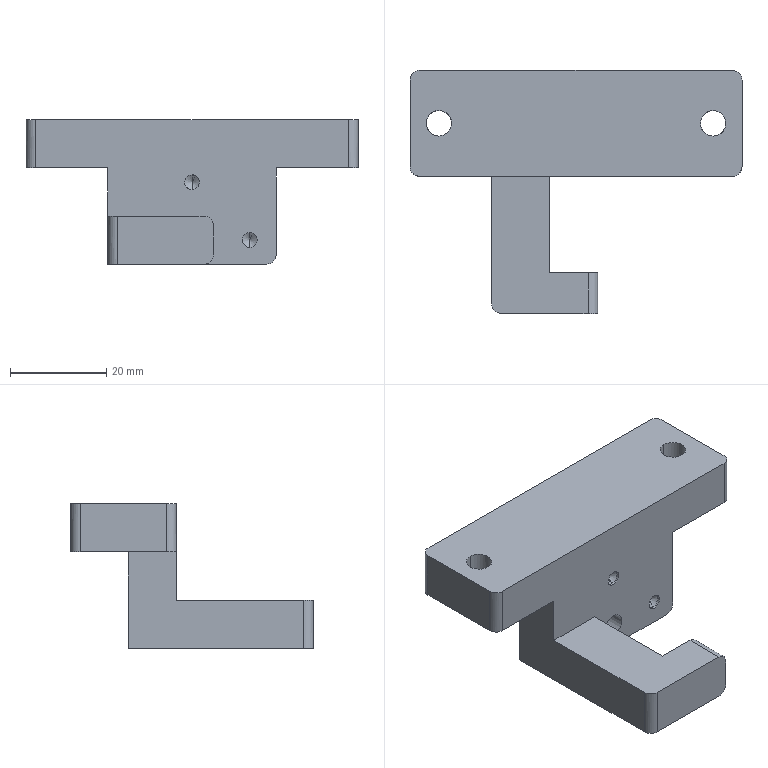NC program | NX | posted with a generic post | part box 69 x 50.5 x 30 mm
Whole program:
N10 G17 G21 G94 G90
(ZLEVEL_PROFILE_1 , TOOL : D10JING)
N12 T14 M6
N14 G54
N16 G17 G0 G90 X-34.145 Y32.098 B0. C0. S9500 M3
N18 G43 Z30. H14
N20 Z-13.5
N22 G94 G1 Z-15. F1000.
N24 X-33.366 Y30.75
N26 G3 X-32.5 Y30.25 R1.
N28 G1 X32.5 F1500.
N30 G2 X39.5 Y23.25 R7.
N32 G1 Y5.25
N34 G2 X32.5 Y-1.75 R7.
N36 G1 X-0.5
N38 Y-11.75
N40 X4.506
N42 G2 X9.5 Y-16.752 R4.998
N44 G1 Y-25.25
N46 G2 X4.5 Y-30.25 R5.
N48 G1 X-15.5
N50 G2 X-22.5 Y-23.25 R7.
N52 G1 Y-1.75
N54 X-32.5
N56 G2 X-39.5 Y5.25 R7.
N58 G1 Y23.25
N60 G2 X-32.5 Y30.25 R7.
N62 G1 X32.5 Z-18.486
N64 X32.866 Y30.24 Z-18.506
N66 X33.232 Y30.212 Z-18.526
N68 X33.595 Y30.164 Z-18.545
N70 X33.955 Y30.097 Z-18.565
N72 X34.312 Y30.011 Z-18.585
N74 X34.663 Y29.907 Z-18.604
N76 X35.009 Y29.785 Z-18.624
N78 X35.347 Y29.645 Z-18.644
N80 X35.678 Y29.487 Z-18.663
N82 X36. Y29.312 Z-18.683
N84 X36.312 Y29.121 Z-18.703
N86 X36.614 Y28.913 Z-18.722
N88 X36.905 Y28.69 Z-18.742
N90 X37.184 Y28.452 Z-18.762
N92 X37.45 Y28.2 Z-18.781
N94 X37.702 Y27.934 Z-18.801
N96 X37.94 Y27.655 Z-18.821
N98 X38.163 Y27.364 Z-18.84
N100 X38.371 Y27.062 Z-18.86
N102 X38.562 Y26.75 Z-18.879
N104 X38.737 Y26.428 Z-18.899
N106 X38.895 Y26.097 Z-18.919
N108 X39.035 Y25.759 Z-18.938
N110 X39.157 Y25.413 Z-18.958
N112 X39.261 Y25.062 Z-18.978
N114 X39.347 Y24.705 Z-18.997
N116 X39.414 Y24.345 Z-19.017
N118 X39.462 Y23.982 Z-19.037
N120 X39.49 Y23.616 Z-19.056
N122 X39.5 Y23.25 Z-19.076
N124 Y5.25 Z-20.041
N126 X39.49 Y4.884 Z-20.061
N128 X39.462 Y4.518 Z-20.081
N130 X39.414 Y4.155 Z-20.1
N132 X39.347 Y3.795 Z-20.12
N134 X39.261 Y3.438 Z-20.14
N136 X39.157 Y3.087 Z-20.159
N138 X39.035 Y2.741 Z-20.179
N140 X38.895 Y2.403 Z-20.199
N142 X38.737 Y2.072 Z-20.218
N144 X38.562 Y1.75 Z-20.238
N146 X38.371 Y1.438 Z-20.258
N148 X38.163 Y1.136 Z-20.277
N150 X37.94 Y0.845 Z-20.297
N152 X37.702 Y0.566 Z-20.317
N154 X37.45 Y0.3 Z-20.336
N156 X37.184 Y0.048 Z-20.356
N158 X36.905 Y-0.19 Z-20.376
N160 X36.614 Y-0.413 Z-20.395
N162 X36.312 Y-0.621 Z-20.415
N164 X36. Y-0.812 Z-20.434
N166 X35.678 Y-0.987 Z-20.454
N168 X35.347 Y-1.145 Z-20.474
N170 X35.009 Y-1.285 Z-20.493
N172 X34.663 Y-1.407 Z-20.513
N174 X34.312 Y-1.511 Z-20.533
N176 X33.955 Y-1.597 Z-20.552
N178 X33.595 Y-1.664 Z-20.572
N180 X33.232 Y-1.712 Z-20.592
N182 X32.866 Y-1.74 Z-20.611
N184 X32.5 Y-1.75 Z-20.631
N186 X-0.5 Z-22.401
N188 Y-11.75 Z-22.937
N190 X2.004 Z-23.072
N192 X4.507 Z-23.206
N194 X4.808 Y-11.76 Z-23.222
N196 X5.109 Y-11.787 Z-23.238
N198 X5.407 Y-11.833 Z-23.255
N200 X5.702 Y-11.897 Z-23.271
N202 X5.993 Y-11.978 Z-23.287
N204 X6.278 Y-12.077 Z-23.303
N206 X6.557 Y-12.193 Z-23.319
N208 X6.828 Y-12.325 Z-23.335
N210 X7.091 Y-12.474 Z-23.352
N212 X7.344 Y-12.638 Z-23.368
N214 X7.587 Y-12.817 Z-23.384
N216 X7.819 Y-13.011 Z-23.4
N218 X8.038 Y-13.218 Z-23.416
N220 X8.245 Y-13.438 Z-23.433
N222 X8.438 Y-13.67 Z-23.449
N224 X8.617 Y-13.913 Z-23.465
N226 X8.781 Y-14.167 Z-23.481
N228 X8.929 Y-14.43 Z-23.497
N230 X9.061 Y-14.701 Z-23.513
N232 X9.176 Y-14.98 Z-23.53
N234 X9.274 Y-15.265 Z-23.546
N236 X9.355 Y-15.556 Z-23.562
N238 X9.418 Y-15.851 Z-23.578
N240 X9.464 Y-16.15 Z-23.594
N242 X9.491 Y-16.45 Z-23.611
N244 X9.5 Y-16.751 Z-23.627
N246 Y-21.001 Z-23.855
N248 Y-25.25 Z-24.083
N250 X9.491 Y-25.552 Z-24.099
N252 X9.464 Y-25.853 Z-24.115
N254 X9.418 Y-26.151 Z-24.131
N256 X9.355 Y-26.447 Z-24.147
N258 X9.274 Y-26.738 Z-24.164
N260 X9.175 Y-27.023 Z-24.18
N262 X9.06 Y-27.302 Z-24.196
N264 X8.927 Y-27.574 Z-24.212
N266 X8.779 Y-27.837 Z-24.228
N268 X8.615 Y-28.09 Z-24.245
N270 X8.436 Y-28.334 Z-24.261
N272 X8.243 Y-28.566 Z-24.277
N274 X8.036 Y-28.786 Z-24.293
N276 X7.816 Y-28.993 Z-24.309
N278 X7.584 Y-29.186 Z-24.325
N280 X7.34 Y-29.365 Z-24.342
N282 X7.087 Y-29.529 Z-24.358
N284 X6.824 Y-29.677 Z-24.374
N286 X6.552 Y-29.81 Z-24.39
N288 X6.273 Y-29.925 Z-24.406
N290 X5.988 Y-30.024 Z-24.423
N292 X5.697 Y-30.105 Z-24.439
N294 X5.401 Y-30.168 Z-24.455
N296 X5.103 Y-30.214 Z-24.471
N298 X4.802 Y-30.241 Z-24.487
N300 X4.5 Y-30.25 Z-24.504
N302 X-15.5 Z-25.576
N304 X-15.866 Y-30.24 Z-25.596
N306 X-16.232 Y-30.212 Z-25.616
N308 X-16.595 Y-30.164 Z-25.635
N310 X-16.955 Y-30.097 Z-25.655
N312 X-17.312 Y-30.011 Z-25.675
N314 X-17.663 Y-29.907 Z-25.694
N316 X-18.009 Y-29.785 Z-25.714
N318 X-18.347 Y-29.645 Z-25.734
N320 X-18.678 Y-29.487 Z-25.753
N322 X-19. Y-29.312 Z-25.773
N324 X-19.312 Y-29.121 Z-25.793
N326 X-19.614 Y-28.913 Z-25.812
N328 X-19.905 Y-28.69 Z-25.832
N330 X-20.184 Y-28.452 Z-25.851
N332 X-20.45 Y-28.2 Z-25.871
N334 X-20.702 Y-27.934 Z-25.891
N336 X-20.94 Y-27.655 Z-25.91
N338 X-21.163 Y-27.364 Z-25.93
N340 X-21.371 Y-27.062 Z-25.95
N342 X-21.562 Y-26.75 Z-25.969
N344 X-21.737 Y-26.428 Z-25.989
N346 X-21.895 Y-26.097 Z-26.009
N348 X-22.035 Y-25.759 Z-26.028
N350 X-22.157 Y-25.413 Z-26.048
N352 X-22.261 Y-25.062 Z-26.068
N354 X-22.347 Y-24.705 Z-26.087
N356 X-22.414 Y-24.345 Z-26.107
N358 X-22.462 Y-23.982 Z-26.127
N360 X-22.49 Y-23.616 Z-26.146
N362 X-22.5 Y-23.25 Z-26.166
N364 Y-1.75 Z-27.319
N366 X-32.5 Z-27.855
N368 X-32.866 Y-1.74 Z-27.875
N370 X-33.232 Y-1.712 Z-27.895
N372 X-33.595 Y-1.664 Z-27.914
N374 X-33.955 Y-1.597 Z-27.934
N376 X-34.312 Y-1.511 Z-27.954
N378 X-34.663 Y-1.407 Z-27.973
N380 X-35.009 Y-1.285 Z-27.993
N382 X-35.347 Y-1.145 Z-28.013
N384 X-35.678 Y-0.987 Z-28.032
N386 X-36. Y-0.812 Z-28.052
N388 X-36.312 Y-0.621 Z-28.072
N390 X-36.614 Y-0.413 Z-28.091
N392 X-36.905 Y-0.19 Z-28.111
N394 X-37.184 Y0.048 Z-28.131
N396 X-37.45 Y0.3 Z-28.15
N398 X-37.702 Y0.566 Z-28.17
N400 X-37.94 Y0.845 Z-28.19
N402 X-38.163 Y1.136 Z-28.209
N404 X-38.371 Y1.438 Z-28.229
N406 X-38.562 Y1.75 Z-28.248
N408 X-38.737 Y2.072 Z-28.268
N410 X-38.895 Y2.403 Z-28.288
N412 X-39.035 Y2.741 Z-28.307
N414 X-39.157 Y3.087 Z-28.327
N416 X-39.261 Y3.438 Z-28.347
N418 X-39.347 Y3.795 Z-28.366
N420 X-39.414 Y4.155 Z-28.386
N422 X-39.462 Y4.518 Z-28.406
N424 X-39.49 Y4.884 Z-28.425
N426 X-39.5 Y5.25 Z-28.445
N428 Y23.25 Z-29.41
N430 X-39.49 Y23.616 Z-29.43
N432 X-39.462 Y23.982 Z-29.45
N434 X-39.414 Y24.345 Z-29.469
N436 X-39.347 Y24.705 Z-29.489
N438 X-39.261 Y25.062 Z-29.509
N440 X-39.157 Y25.413 Z-29.528
N442 X-39.035 Y25.759 Z-29.548
N444 X-38.895 Y26.097 Z-29.568
N446 X-38.737 Y26.428 Z-29.587
N448 X-38.562 Y26.75 Z-29.607
N450 X-38.371 Y27.062 Z-29.627
N452 X-38.163 Y27.364 Z-29.646
N454 X-37.94 Y27.655 Z-29.666
N456 X-37.702 Y27.934 Z-29.686
N458 X-37.45 Y28.2 Z-29.705
N460 X-37.184 Y28.452 Z-29.725
N462 X-36.905 Y28.69 Z-29.745
N464 X-36.614 Y28.913 Z-29.764
N466 X-36.312 Y29.121 Z-29.784
N468 X-36. Y29.312 Z-29.803
N470 X-35.678 Y29.487 Z-29.823
N472 X-35.347 Y29.645 Z-29.843
N474 X-35.009 Y29.785 Z-29.862
N476 X-34.663 Y29.907 Z-29.882
N478 X-34.312 Y30.011 Z-29.902
N480 X-33.955 Y30.097 Z-29.921
N482 X-33.595 Y30.164 Z-29.941
N484 X-33.232 Y30.212 Z-29.961
N486 X-32.866 Y30.24 Z-29.98
N488 X-32.5 Y30.25 Z-30.
N490 X32.5
N492 G2 X39.5 Y23.25 R7.
N494 G1 Y5.25
N496 G2 X32.5 Y-1.75 R7.
N498 G1 X-0.5
N500 Y-11.75
N502 X4.507
N504 G2 X9.5 Y-16.752 R4.998
N506 G1 Y-25.25
N508 G2 X4.5 Y-30.25 R5.
N510 G1 X-15.5
N512 G2 X-22.5 Y-23.25 R7.
N514 G1 Y-1.75
N516 X-32.5
N518 G2 X-39.5 Y5.25 R7.
N520 G1 Y23.25
N522 G2 X-32.5 Y30.25 R7.
N524 G3 X-31.634 Y30.75 R1.
N526 G1 X-30.768 Y32.25
N528 Z-28.5
N530 G0 Z30.
N532 M5
(FLOOR_WALL_1_COPY , TOOL : D6)
N534 T12 M6
N536 G54
N538 G17 G0 G90 X-22. Y-15.362 B0. C0. S9500 M3
N540 G43 Z30. H12
N542 Z-18.5
N544 G94 G1 Z-20. F1200.
N546 X-20.8 Y-14.67
N548 G3 X-20.5 Y-14.15 R0.6
N550 G1 Y-0.05
N552 X-2.5
N554 Y-13.75
N556 X5.5
N558 Y-28.25
N560 X-15.637
N562 X-16.42 Y-28.178
N564 X-17.352 Y-27.91
N566 X-18.247 Y-27.446
N568 X-19.047 Y-26.797
N570 X-19.696 Y-25.997
N572 X-20.16 Y-25.102
N574 X-20.428 Y-24.17
N576 X-20.5 Y-23.387
N578 Y-14.15
N580 X-17.5
N582 Y-3.05
N584 X-5.5
N586 Y-13.75
N588 G3 X-2.5 Y-16.75 R3.
N590 G1 X2.5
N592 Y-25.25
N594 X-15.5
N596 G2 X-17.5 Y-23.25 R2.
N598 G1 Y-14.15
N600 X-14.5
N602 Y-6.05
N604 X-8.5
N606 Y-13.75
N608 G3 X-2.5 Y-19.75 R6.
N610 G1 X-0.5
N612 Y-22.25
N614 X-14.5
N616 Y-14.15
N618 X-11.5
N620 Y-9.05
N622 Y-13.75
N624 G3 X-9.624 Y-19.25 R9.
N626 G1 X-11.5
N628 Y-14.15
N630 G3 X-11.8 Y-13.63 R0.6
N632 G1 Z-18.5
N634 G0 X-1. Y-1.748
N636 G1 Z-20.
N638 X-1.98 Y-0.05
N640 G3 X-2.5 Y0.25 R0.6
N642 G1 X-20.5
N644 G3 X-21.02 Y-0.05 R0.6
N646 G1 X-22. Y-1.748
N648 Z-18.5
N650 G0 Z30.
(PLANAR_MILL_COPY , TOOL : D6A45)
N652 T01 M6
N654 G17 G43 G0 G90 X29.75 Y13.384 Z30. B0. C0. S9500 H1 M3
N656 Z0.5
N658 G94 G1 Z-1. F1250.
N660 G3 X30.25 Y14.25 R1.
N662 X28.5 Y16. R1.75
N664 X30.25 Y14.25 R-1.75
N666 X29.75 Y15.116 R1.
N668 G1 Z0.5
N670 G0 Z30.
N672 X-0.866 Y26.65
N674 Z0.5
N676 G1 Z-1.
N678 G3 X0. Y26.15 R1.
N680 G1 X32.5
N682 G2 X35.4 Y23.25 R2.9
N684 G1 Y5.25
N686 G2 X32.5 Y2.35 R2.9
N688 G1 X-32.5
N690 G2 X-35.4 Y5.25 R2.9
N692 G1 Y23.25
N694 G2 X-32.5 Y26.15 R2.9
N696 G1 X0.
N698 G3 X0.866 Y26.65 R1.
N700 G1 Z0.5
N702 G0 Z30.
N704 X-29.75 Y15.116
N706 Z0.5
N708 G1 Z-1.
N710 G3 X-30.25 Y14.25 R1.
N712 X-28.5 Y12.5 R1.75
N714 X-30.25 Y14.25 R-1.75
N716 X-29.75 Y13.384 R1.
N718 G1 Z0.5
N720 G0 Z30.
N722 M5
N724 M2